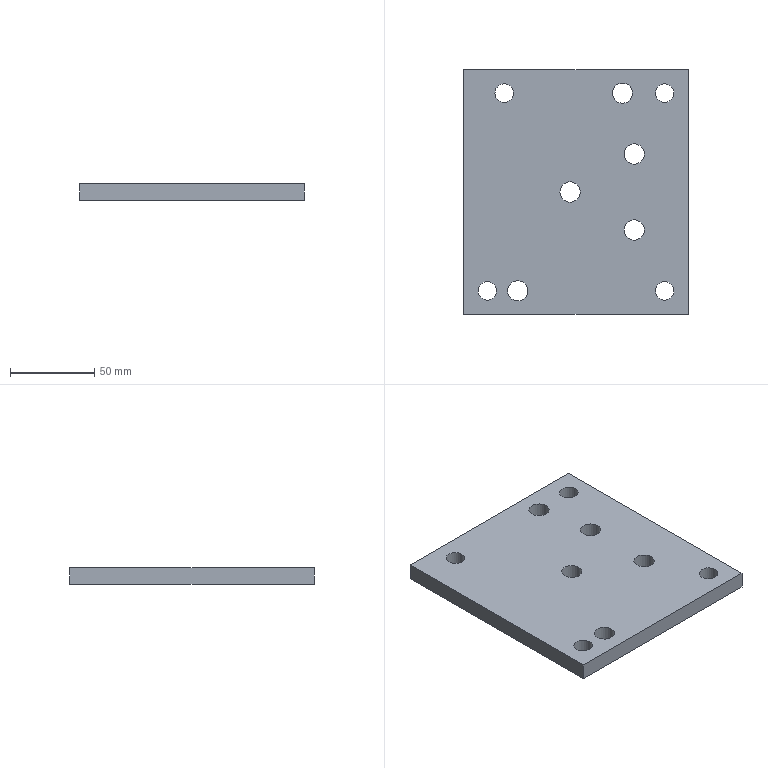Part | STEP file | lll_id2986_x_t | 1 solid | 15 faces | box 133 x 145 x 10 mm | volume 183394 mm3 | cylinder 9 | plane 6 | commonest cylinder face diameters 12 x5 11 x4
STEP:
#1=CARTESIAN_POINT('',(3864.,58.5,102.5));
#2=VERTEX_POINT('',#1);
#3=CARTESIAN_POINT('',(3870.,58.5,102.5));
#4=DIRECTION('',(0.,0.,-1.));
#5=DIRECTION('',(-1.,0.,0.));
#6=AXIS2_PLACEMENT_3D('',#3,#4,#5);
#7=CIRCLE('',#6,6.);
#8=EDGE_CURVE('',#2,#2,#7,.T.);
#9=ORIENTED_EDGE('',*,*,#8,.F.);
#10=EDGE_LOOP('',(#9));
#11=FACE_BOUND('',#10,.T.);
#12=CARTESIAN_POINT('',(3864.,58.5,92.5));
#13=VERTEX_POINT('',#12);
#14=CARTESIAN_POINT('',(3870.,58.5,92.5));
#15=DIRECTION('',(0.,0.,1.));
#16=DIRECTION('',(-1.,0.,0.));
#17=AXIS2_PLACEMENT_3D('',#14,#15,#16);
#18=CIRCLE('',#17,6.);
#19=EDGE_CURVE('',#13,#13,#18,.T.);
#20=ORIENTED_EDGE('',*,*,#19,.F.);
#21=EDGE_LOOP('',(#20));
#22=FACE_BOUND('',#21,.T.);
#23=CARTESIAN_POINT('',(3870.,58.5,92.5));
#24=DIRECTION('',(0.,0.,1.));
#25=DIRECTION('',(-1.,0.,0.));
#26=AXIS2_PLACEMENT_3D('',#23,#24,#25);
#27=CYLINDRICAL_SURFACE('',#26,6.);
#28=ADVANCED_FACE('',(#11,#22),#27,.F.);
#29=CARTESIAN_POINT('',(3794.5,58.5,102.5));
#30=VERTEX_POINT('',#29);
#31=CARTESIAN_POINT('',(3800.,58.5,102.5));
#32=DIRECTION('',(0.,0.,-1.));
#33=DIRECTION('',(-1.,0.,0.));
#34=AXIS2_PLACEMENT_3D('',#31,#32,#33);
#35=CIRCLE('',#34,5.5);
#36=EDGE_CURVE('',#30,#30,#35,.T.);
#37=ORIENTED_EDGE('',*,*,#36,.F.);
#38=EDGE_LOOP('',(#37));
#39=FACE_BOUND('',#38,.T.);
#40=CARTESIAN_POINT('',(3805.5,58.5,92.5));
#41=VERTEX_POINT('',#40);
#42=CARTESIAN_POINT('',(3800.,58.5,92.5));
#43=DIRECTION('',(0.,0.,1.));
#44=DIRECTION('',(1.,0.,0.));
#45=AXIS2_PLACEMENT_3D('',#42,#43,#44);
#46=CIRCLE('',#45,5.5);
#47=EDGE_CURVE('',#41,#41,#46,.T.);
#48=ORIENTED_EDGE('',*,*,#47,.F.);
#49=EDGE_LOOP('',(#48));
#50=FACE_BOUND('',#49,.T.);
#51=CARTESIAN_POINT('',(3800.,58.5,92.5));
#52=DIRECTION('',(0.,0.,1.));
#53=DIRECTION('',(-1.,0.,0.));
#54=AXIS2_PLACEMENT_3D('',#51,#52,#53);
#55=CYLINDRICAL_SURFACE('',#54,5.5);
#56=ADVANCED_FACE('',(#39,#50),#55,.F.);
#57=CARTESIAN_POINT('',(3889.5,58.5,102.5));
#58=VERTEX_POINT('',#57);
#59=CARTESIAN_POINT('',(3895.,58.5,102.5));
#60=DIRECTION('',(0.,0.,1.));
#61=DIRECTION('',(-1.,0.,0.));
#62=AXIS2_PLACEMENT_3D('',#59,#60,#61);
#63=CIRCLE('',#62,5.5);
#64=EDGE_CURVE('',#58,#58,#63,.T.);
#65=ORIENTED_EDGE('',*,*,#64,.T.);
#66=EDGE_LOOP('',(#65));
#67=FACE_BOUND('',#66,.T.);
#68=CARTESIAN_POINT('',(3900.5,58.5,92.5));
#69=VERTEX_POINT('',#68);
#70=CARTESIAN_POINT('',(3895.,58.5,92.5));
#71=DIRECTION('',(0.,0.,1.));
#72=DIRECTION('',(1.,0.,0.));
#73=AXIS2_PLACEMENT_3D('',#70,#71,#72);
#74=CIRCLE('',#73,5.5);
#75=EDGE_CURVE('',#69,#69,#74,.T.);
#76=ORIENTED_EDGE('',*,*,#75,.F.);
#77=EDGE_LOOP('',(#76));
#78=FACE_BOUND('',#77,.T.);
#79=CARTESIAN_POINT('',(3895.,58.5,92.5));
#80=DIRECTION('',(0.,0.,1.));
#81=DIRECTION('',(-1.,0.,0.));
#82=AXIS2_PLACEMENT_3D('',#79,#80,#81);
#83=CYLINDRICAL_SURFACE('',#82,5.5);
#84=ADVANCED_FACE('',(#67,#78),#83,.F.);
#85=CARTESIAN_POINT('',(3776.,72.5,102.5));
#86=VERTEX_POINT('',#85);
#87=CARTESIAN_POINT('',(3776.,-72.5,102.5));
#88=VERTEX_POINT('',#87);
#89=CARTESIAN_POINT('',(3776.,0.00007613,102.5));
#90=DIRECTION('',(0.,-1.,0.));
#91=VECTOR('',#90,1.);
#92=LINE('',#89,#91);
#93=EDGE_CURVE('',#86,#88,#92,.T.);
#94=ORIENTED_EDGE('',*,*,#93,.F.);
#95=CARTESIAN_POINT('',(3776.,72.5,92.5));
#96=VERTEX_POINT('',#95);
#97=CARTESIAN_POINT('',(3776.,72.5,92.5));
#98=DIRECTION('',(0.,0.,1.));
#99=VECTOR('',#98,1.);
#100=LINE('',#97,#99);
#101=EDGE_CURVE('',#96,#86,#100,.T.);
#102=ORIENTED_EDGE('',*,*,#101,.F.);
#103=CARTESIAN_POINT('',(3776.,-72.5,92.5));
#104=VERTEX_POINT('',#103);
#105=CARTESIAN_POINT('',(3776.,0.00007613,92.5));
#106=DIRECTION('',(0.,-1.,0.));
#107=VECTOR('',#106,1.);
#108=LINE('',#105,#107);
#109=EDGE_CURVE('',#96,#104,#108,.T.);
#110=ORIENTED_EDGE('',*,*,#109,.T.);
#111=CARTESIAN_POINT('',(3776.,-72.5,92.5));
#112=DIRECTION('',(0.,0.,1.));
#113=VECTOR('',#112,1.);
#114=LINE('',#111,#113);
#115=EDGE_CURVE('',#104,#88,#114,.T.);
#116=ORIENTED_EDGE('',*,*,#115,.T.);
#117=EDGE_LOOP('',(#94,#102,#110,#116));
#118=FACE_OUTER_BOUND('',#117,.T.);
#119=CARTESIAN_POINT('',(3776.,0.00007613,92.5));
#120=DIRECTION('',(-1.,0.,0.));
#121=DIRECTION('',(0.,0.,-1.));
#122=AXIS2_PLACEMENT_3D('',#119,#120,#121);
#123=PLANE('',#122);
#124=ADVANCED_FACE('',(#118),#123,.T.);
#125=CARTESIAN_POINT('',(3909.,-72.5,102.5));
#126=VERTEX_POINT('',#125);
#127=CARTESIAN_POINT('',(3841.5,-72.5,102.5));
#128=DIRECTION('',(1.,0.,0.));
#129=VECTOR('',#128,1.);
#130=LINE('',#127,#129);
#131=EDGE_CURVE('',#88,#126,#130,.T.);
#132=ORIENTED_EDGE('',*,*,#131,.F.);
#133=ORIENTED_EDGE('',*,*,#115,.F.);
#134=CARTESIAN_POINT('',(3909.,-72.5,92.5));
#135=VERTEX_POINT('',#134);
#136=CARTESIAN_POINT('',(3841.5,-72.5,92.5));
#137=DIRECTION('',(1.,0.,0.));
#138=VECTOR('',#137,1.);
#139=LINE('',#136,#138);
#140=EDGE_CURVE('',#104,#135,#139,.T.);
#141=ORIENTED_EDGE('',*,*,#140,.T.);
#142=CARTESIAN_POINT('',(3909.,-72.5,92.5));
#143=DIRECTION('',(0.,0.,1.));
#144=VECTOR('',#143,1.);
#145=LINE('',#142,#144);
#146=EDGE_CURVE('',#135,#126,#145,.T.);
#147=ORIENTED_EDGE('',*,*,#146,.T.);
#148=EDGE_LOOP('',(#132,#133,#141,#147));
#149=FACE_OUTER_BOUND('',#148,.T.);
#150=CARTESIAN_POINT('',(3841.5,-72.5,92.5));
#151=DIRECTION('',(0.,-1.,0.));
#152=DIRECTION('',(0.,0.,1.));
#153=AXIS2_PLACEMENT_3D('',#150,#151,#152);
#154=PLANE('',#153);
#155=ADVANCED_FACE('',(#149),#154,.T.);
#156=CARTESIAN_POINT('',(3909.,72.5,102.5));
#157=VERTEX_POINT('',#156);
#158=CARTESIAN_POINT('',(3909.,0.00007613,102.5));
#159=DIRECTION('',(0.,1.,0.));
#160=VECTOR('',#159,1.);
#161=LINE('',#158,#160);
#162=EDGE_CURVE('',#126,#157,#161,.T.);
#163=ORIENTED_EDGE('',*,*,#162,.F.);
#164=ORIENTED_EDGE('',*,*,#146,.F.);
#165=CARTESIAN_POINT('',(3909.,72.5,92.5));
#166=VERTEX_POINT('',#165);
#167=CARTESIAN_POINT('',(3909.,0.00007613,92.5));
#168=DIRECTION('',(0.,1.,0.));
#169=VECTOR('',#168,1.);
#170=LINE('',#167,#169);
#171=EDGE_CURVE('',#135,#166,#170,.T.);
#172=ORIENTED_EDGE('',*,*,#171,.T.);
#173=CARTESIAN_POINT('',(3909.,72.5,92.5));
#174=DIRECTION('',(0.,0.,1.));
#175=VECTOR('',#174,1.);
#176=LINE('',#173,#175);
#177=EDGE_CURVE('',#166,#157,#176,.T.);
#178=ORIENTED_EDGE('',*,*,#177,.T.);
#179=EDGE_LOOP('',(#163,#164,#172,#178));
#180=FACE_OUTER_BOUND('',#179,.T.);
#181=CARTESIAN_POINT('',(3909.,0.00007613,92.5));
#182=DIRECTION('',(1.,0.,0.));
#183=DIRECTION('',(0.,0.,1.));
#184=AXIS2_PLACEMENT_3D('',#181,#182,#183);
#185=PLANE('',#184);
#186=ADVANCED_FACE('',(#180),#185,.T.);
#187=CARTESIAN_POINT('',(3841.5,72.5,102.5));
#188=DIRECTION('',(-1.,0.,0.));
#189=VECTOR('',#188,1.);
#190=LINE('',#187,#189);
#191=EDGE_CURVE('',#157,#86,#190,.T.);
#192=ORIENTED_EDGE('',*,*,#191,.F.);
#193=ORIENTED_EDGE('',*,*,#177,.F.);
#194=CARTESIAN_POINT('',(3841.5,72.5,92.5));
#195=DIRECTION('',(-1.,0.,0.));
#196=VECTOR('',#195,1.);
#197=LINE('',#194,#196);
#198=EDGE_CURVE('',#166,#96,#197,.T.);
#199=ORIENTED_EDGE('',*,*,#198,.T.);
#200=ORIENTED_EDGE('',*,*,#101,.T.);
#201=EDGE_LOOP('',(#192,#193,#199,#200));
#202=FACE_OUTER_BOUND('',#201,.T.);
#203=CARTESIAN_POINT('',(3841.5,72.5,92.5));
#204=DIRECTION('',(0.,1.,0.));
#205=DIRECTION('',(0.,0.,-1.));
#206=AXIS2_PLACEMENT_3D('',#203,#204,#205);
#207=PLANE('',#206);
#208=ADVANCED_FACE('',(#202),#207,.T.);
#209=CARTESIAN_POINT('',(3784.5,-58.5,102.5));
#210=VERTEX_POINT('',#209);
#211=CARTESIAN_POINT('',(3790.,-58.5,102.5));
#212=DIRECTION('',(0.,0.,1.));
#213=DIRECTION('',(-1.,0.,0.));
#214=AXIS2_PLACEMENT_3D('',#211,#212,#213);
#215=CIRCLE('',#214,5.5);
#216=EDGE_CURVE('',#210,#210,#215,.T.);
#217=ORIENTED_EDGE('',*,*,#216,.T.);
#218=EDGE_LOOP('',(#217));
#219=FACE_BOUND('',#218,.T.);
#220=CARTESIAN_POINT('',(3795.5,-58.5,92.5));
#221=VERTEX_POINT('',#220);
#222=CARTESIAN_POINT('',(3790.,-58.5,92.5));
#223=DIRECTION('',(0.,0.,1.));
#224=DIRECTION('',(1.,0.,0.));
#225=AXIS2_PLACEMENT_3D('',#222,#223,#224);
#226=CIRCLE('',#225,5.5);
#227=EDGE_CURVE('',#221,#221,#226,.T.);
#228=ORIENTED_EDGE('',*,*,#227,.F.);
#229=EDGE_LOOP('',(#228));
#230=FACE_BOUND('',#229,.T.);
#231=CARTESIAN_POINT('',(3790.,-58.5,92.5));
#232=DIRECTION('',(0.,0.,1.));
#233=DIRECTION('',(-1.,0.,0.));
#234=AXIS2_PLACEMENT_3D('',#231,#232,#233);
#235=CYLINDRICAL_SURFACE('',#234,5.5);
#236=ADVANCED_FACE('',(#219,#230),#235,.F.);
#237=CARTESIAN_POINT('',(3889.5,-58.5,102.5));
#238=VERTEX_POINT('',#237);
#239=CARTESIAN_POINT('',(3895.,-58.5,102.5));
#240=DIRECTION('',(0.,0.,1.));
#241=DIRECTION('',(-1.,0.,0.));
#242=AXIS2_PLACEMENT_3D('',#239,#240,#241);
#243=CIRCLE('',#242,5.5);
#244=EDGE_CURVE('',#238,#238,#243,.T.);
#245=ORIENTED_EDGE('',*,*,#244,.T.);
#246=EDGE_LOOP('',(#245));
#247=FACE_BOUND('',#246,.T.);
#248=CARTESIAN_POINT('',(3900.5,-58.5,92.5));
#249=VERTEX_POINT('',#248);
#250=CARTESIAN_POINT('',(3895.,-58.5,92.5));
#251=DIRECTION('',(0.,0.,1.));
#252=DIRECTION('',(1.,0.,0.));
#253=AXIS2_PLACEMENT_3D('',#250,#251,#252);
#254=CIRCLE('',#253,5.5);
#255=EDGE_CURVE('',#249,#249,#254,.T.);
#256=ORIENTED_EDGE('',*,*,#255,.F.);
#257=EDGE_LOOP('',(#256));
#258=FACE_BOUND('',#257,.T.);
#259=CARTESIAN_POINT('',(3895.,-58.5,92.5));
#260=DIRECTION('',(0.,0.,1.));
#261=DIRECTION('',(-1.,0.,0.));
#262=AXIS2_PLACEMENT_3D('',#259,#260,#261);
#263=CYLINDRICAL_SURFACE('',#262,5.5);
#264=ADVANCED_FACE('',(#247,#258),#263,.F.);
#265=CARTESIAN_POINT('',(3871.,22.5,92.5));
#266=VERTEX_POINT('',#265);
#267=CARTESIAN_POINT('',(3877.,22.5,92.5));
#268=DIRECTION('',(0.,0.,-1.));
#269=DIRECTION('',(-1.,0.,0.));
#270=AXIS2_PLACEMENT_3D('',#267,#268,#269);
#271=CIRCLE('',#270,6.);
#272=EDGE_CURVE('',#266,#266,#271,.T.);
#273=ORIENTED_EDGE('',*,*,#272,.F.);
#274=EDGE_LOOP('',(#273));
#275=FACE_BOUND('',#274,.T.);
#276=CARTESIAN_POINT('',(3832.982,-0.01982,92.5));
#277=VERTEX_POINT('',#276);
#278=CARTESIAN_POINT('',(3838.982,-0.01982,92.5));
#279=DIRECTION('',(0.,0.,-1.));
#280=DIRECTION('',(-1.,0.,0.));
#281=AXIS2_PLACEMENT_3D('',#278,#279,#280);
#282=CIRCLE('',#281,6.);
#283=EDGE_CURVE('',#277,#277,#282,.T.);
#284=ORIENTED_EDGE('',*,*,#283,.F.);
#285=EDGE_LOOP('',(#284));
#286=FACE_BOUND('',#285,.T.);
#287=CARTESIAN_POINT('',(3870.982,-22.52,92.5));
#288=VERTEX_POINT('',#287);
#289=CARTESIAN_POINT('',(3876.982,-22.52,92.5));
#290=DIRECTION('',(0.,0.,-1.));
#291=DIRECTION('',(-1.,0.,0.));
#292=AXIS2_PLACEMENT_3D('',#289,#290,#291);
#293=CIRCLE('',#292,6.);
#294=EDGE_CURVE('',#288,#288,#293,.T.);
#295=ORIENTED_EDGE('',*,*,#294,.F.);
#296=EDGE_LOOP('',(#295));
#297=FACE_BOUND('',#296,.T.);
#298=CARTESIAN_POINT('',(3802.,-58.5,92.5));
#299=VERTEX_POINT('',#298);
#300=CARTESIAN_POINT('',(3808.,-58.5,92.5));
#301=DIRECTION('',(0.,0.,1.));
#302=DIRECTION('',(-1.,0.,0.));
#303=AXIS2_PLACEMENT_3D('',#300,#301,#302);
#304=CIRCLE('',#303,6.);
#305=EDGE_CURVE('',#299,#299,#304,.T.);
#306=ORIENTED_EDGE('',*,*,#305,.T.);
#307=EDGE_LOOP('',(#306));
#308=FACE_BOUND('',#307,.T.);
#309=ORIENTED_EDGE('',*,*,#255,.T.);
#310=EDGE_LOOP('',(#309));
#311=FACE_BOUND('',#310,.T.);
#312=ORIENTED_EDGE('',*,*,#227,.T.);
#313=EDGE_LOOP('',(#312));
#314=FACE_BOUND('',#313,.T.);
#315=ORIENTED_EDGE('',*,*,#109,.F.);
#316=ORIENTED_EDGE('',*,*,#198,.F.);
#317=ORIENTED_EDGE('',*,*,#171,.F.);
#318=ORIENTED_EDGE('',*,*,#140,.F.);
#319=EDGE_LOOP('',(#315,#316,#317,#318));
#320=FACE_BOUND('',#319,.T.);
#321=ORIENTED_EDGE('',*,*,#75,.T.);
#322=EDGE_LOOP('',(#321));
#323=FACE_BOUND('',#322,.T.);
#324=ORIENTED_EDGE('',*,*,#47,.T.);
#325=EDGE_LOOP('',(#324));
#326=FACE_BOUND('',#325,.T.);
#327=ORIENTED_EDGE('',*,*,#19,.T.);
#328=EDGE_LOOP('',(#327));
#329=FACE_BOUND('',#328,.T.);
#330=CARTESIAN_POINT('',(3841.5,0.00007613,92.5));
#331=DIRECTION('',(0.,0.,-1.));
#332=DIRECTION('',(1.,0.,0.));
#333=AXIS2_PLACEMENT_3D('',#330,#331,#332);
#334=PLANE('',#333);
#335=ADVANCED_FACE('',(#275,#286,#297,#308,#311,#314,#320,#323,#326,#329),#334,.T.);
#336=CARTESIAN_POINT('',(3802.,-58.5,102.5));
#337=VERTEX_POINT('',#336);
#338=CARTESIAN_POINT('',(3808.,-58.5,102.5));
#339=DIRECTION('',(0.,0.,1.));
#340=DIRECTION('',(-1.,0.,0.));
#341=AXIS2_PLACEMENT_3D('',#338,#339,#340);
#342=CIRCLE('',#341,6.);
#343=EDGE_CURVE('',#337,#337,#342,.T.);
#344=ORIENTED_EDGE('',*,*,#343,.T.);
#345=EDGE_LOOP('',(#344));
#346=FACE_BOUND('',#345,.T.);
#347=ORIENTED_EDGE('',*,*,#305,.F.);
#348=EDGE_LOOP('',(#347));
#349=FACE_BOUND('',#348,.T.);
#350=CARTESIAN_POINT('',(3808.,-58.5,92.5));
#351=DIRECTION('',(0.,0.,1.));
#352=DIRECTION('',(-1.,0.,0.));
#353=AXIS2_PLACEMENT_3D('',#350,#351,#352);
#354=CYLINDRICAL_SURFACE('',#353,6.);
#355=ADVANCED_FACE('',(#346,#349),#354,.F.);
#356=CARTESIAN_POINT('',(3871.,22.5,102.5));
#357=VERTEX_POINT('',#356);
#358=CARTESIAN_POINT('',(3877.,22.5,102.5));
#359=DIRECTION('',(0.,0.,-1.));
#360=DIRECTION('',(-1.,0.,0.));
#361=AXIS2_PLACEMENT_3D('',#358,#359,#360);
#362=CIRCLE('',#361,6.);
#363=EDGE_CURVE('',#357,#357,#362,.T.);
#364=ORIENTED_EDGE('',*,*,#363,.T.);
#365=EDGE_LOOP('',(#364));
#366=FACE_BOUND('',#365,.T.);
#367=CARTESIAN_POINT('',(3832.982,-0.01982,102.5));
#368=VERTEX_POINT('',#367);
#369=CARTESIAN_POINT('',(3838.982,-0.01982,102.5));
#370=DIRECTION('',(0.,0.,-1.));
#371=DIRECTION('',(-1.,0.,0.));
#372=AXIS2_PLACEMENT_3D('',#369,#370,#371);
#373=CIRCLE('',#372,6.);
#374=EDGE_CURVE('',#368,#368,#373,.T.);
#375=ORIENTED_EDGE('',*,*,#374,.T.);
#376=EDGE_LOOP('',(#375));
#377=FACE_BOUND('',#376,.T.);
#378=CARTESIAN_POINT('',(3870.982,-22.52,102.5));
#379=VERTEX_POINT('',#378);
#380=CARTESIAN_POINT('',(3876.982,-22.52,102.5));
#381=DIRECTION('',(0.,0.,-1.));
#382=DIRECTION('',(-1.,0.,0.));
#383=AXIS2_PLACEMENT_3D('',#380,#381,#382);
#384=CIRCLE('',#383,6.);
#385=EDGE_CURVE('',#379,#379,#384,.T.);
#386=ORIENTED_EDGE('',*,*,#385,.T.);
#387=EDGE_LOOP('',(#386));
#388=FACE_BOUND('',#387,.T.);
#389=ORIENTED_EDGE('',*,*,#191,.T.);
#390=ORIENTED_EDGE('',*,*,#93,.T.);
#391=ORIENTED_EDGE('',*,*,#131,.T.);
#392=ORIENTED_EDGE('',*,*,#162,.T.);
#393=EDGE_LOOP('',(#389,#390,#391,#392));
#394=FACE_BOUND('',#393,.T.);
#395=ORIENTED_EDGE('',*,*,#216,.F.);
#396=EDGE_LOOP('',(#395));
#397=FACE_BOUND('',#396,.T.);
#398=ORIENTED_EDGE('',*,*,#244,.F.);
#399=EDGE_LOOP('',(#398));
#400=FACE_BOUND('',#399,.T.);
#401=ORIENTED_EDGE('',*,*,#343,.F.);
#402=EDGE_LOOP('',(#401));
#403=FACE_BOUND('',#402,.T.);
#404=ORIENTED_EDGE('',*,*,#8,.T.);
#405=EDGE_LOOP('',(#404));
#406=FACE_BOUND('',#405,.T.);
#407=ORIENTED_EDGE('',*,*,#36,.T.);
#408=EDGE_LOOP('',(#407));
#409=FACE_BOUND('',#408,.T.);
#410=ORIENTED_EDGE('',*,*,#64,.F.);
#411=EDGE_LOOP('',(#410));
#412=FACE_BOUND('',#411,.T.);
#413=CARTESIAN_POINT('',(3312.867,136.288,102.5));
#414=DIRECTION('',(0.,0.,-1.));
#415=DIRECTION('',(-1.,0.,0.));
#416=AXIS2_PLACEMENT_3D('',#413,#414,#415);
#417=PLANE('',#416);
#418=ADVANCED_FACE('',(#366,#377,#388,#394,#397,#400,#403,#406,#409,#412),#417,.F.);
#419=ORIENTED_EDGE('',*,*,#294,.T.);
#420=EDGE_LOOP('',(#419));
#421=FACE_BOUND('',#420,.T.);
#422=ORIENTED_EDGE('',*,*,#385,.F.);
#423=EDGE_LOOP('',(#422));
#424=FACE_BOUND('',#423,.T.);
#425=CARTESIAN_POINT('',(3876.982,-22.52,62.5));
#426=DIRECTION('',(0.,0.,1.));
#427=DIRECTION('',(-1.,0.,0.));
#428=AXIS2_PLACEMENT_3D('',#425,#426,#427);
#429=CYLINDRICAL_SURFACE('',#428,6.);
#430=ADVANCED_FACE('',(#421,#424),#429,.F.);
#431=ORIENTED_EDGE('',*,*,#283,.T.);
#432=EDGE_LOOP('',(#431));
#433=FACE_BOUND('',#432,.T.);
#434=ORIENTED_EDGE('',*,*,#374,.F.);
#435=EDGE_LOOP('',(#434));
#436=FACE_BOUND('',#435,.T.);
#437=CARTESIAN_POINT('',(3838.982,-0.01982,62.5));
#438=DIRECTION('',(0.,0.,1.));
#439=DIRECTION('',(-1.,0.,0.));
#440=AXIS2_PLACEMENT_3D('',#437,#438,#439);
#441=CYLINDRICAL_SURFACE('',#440,6.);
#442=ADVANCED_FACE('',(#433,#436),#441,.F.);
#443=ORIENTED_EDGE('',*,*,#272,.T.);
#444=EDGE_LOOP('',(#443));
#445=FACE_BOUND('',#444,.T.);
#446=ORIENTED_EDGE('',*,*,#363,.F.);
#447=EDGE_LOOP('',(#446));
#448=FACE_BOUND('',#447,.T.);
#449=CARTESIAN_POINT('',(3877.,22.5,62.5));
#450=DIRECTION('',(0.,0.,1.));
#451=DIRECTION('',(-1.,0.,0.));
#452=AXIS2_PLACEMENT_3D('',#449,#450,#451);
#453=CYLINDRICAL_SURFACE('',#452,6.);
#454=ADVANCED_FACE('',(#445,#448),#453,.F.);
#455=CLOSED_SHELL('',(#28,#56,#84,#124,#155,#186,#208,#236,#264,#335,#355,#418,#430,#442,#454));
#456=MANIFOLD_SOLID_BREP('',#455);
#457=(LENGTH_UNIT()NAMED_UNIT(*)SI_UNIT(.MILLI.,.METRE.));
#458=UNCERTAINTY_MEASURE_WITH_UNIT(LENGTH_MEASURE(0.00002),#457,'','');
#459=(NAMED_UNIT(*)PLANE_ANGLE_UNIT()SI_UNIT($,.RADIAN.));
#460=PLANE_ANGLE_MEASURE_WITH_UNIT(PLANE_ANGLE_MEASURE(0.01745),#459);
#461=DIMENSIONAL_EXPONENTS(0.,0.,0.,0.,0.,0.,0.);
#462=(CONVERSION_BASED_UNIT('DEGREE',#460)NAMED_UNIT(#461)PLANE_ANGLE_UNIT());
#463=(NAMED_UNIT(*)SI_UNIT($,.STERADIAN.)SOLID_ANGLE_UNIT());
#464=(GEOMETRIC_REPRESENTATION_CONTEXT(3)GLOBAL_UNCERTAINTY_ASSIGNED_CONTEXT((#458))GLOBAL_UNIT_ASSIGNED_CONTEXT((#457,#462,#463))REPRESENTATION_CONTEXT('',''));
#465=ADVANCED_BREP_SHAPE_REPRESENTATION('',(#456),#464);